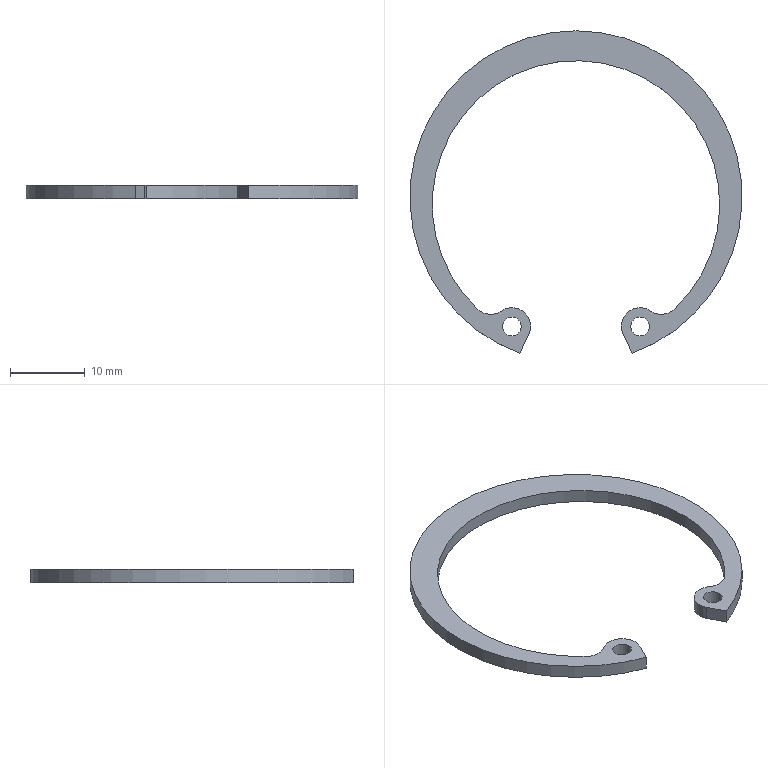Part | STEP file | KS B 1336 - 42x1.8 | 1 solid | 16 faces | box 44.5 x 43.174 x 1.8 mm | volume 686.31 mm3 | cylinder 12 | plane 4 | commonest cylinder face diameters 2.5 x4 5 x4 38.5 x2 44.5 x2
STEP:
#1=CARTESIAN_POINT('',(0.,0.,0.));
#2=DIRECTION('',(0.,0.,1.));
#3=DIRECTION('',(1.,0.,0.));
#4=AXIS2_PLACEMENT_3D('',#1,#2,#3);
#5=CARTESIAN_POINT('',(7.332,-38.343,0.));
#6=VERTEX_POINT('',#5);
#7=CARTESIAN_POINT('',(7.332,-38.343,1.8));
#8=VERTEX_POINT('',#7);
#9=CARTESIAN_POINT('',(7.332,-38.343,0.));
#10=DIRECTION('',(0.,0.,1.));
#11=VECTOR('',#10,1.);
#12=LINE('',#9,#11);
#13=CARTESIAN_POINT('',(8.582,-38.343,0.));
#14=DIRECTION('',(0.,0.,1.));
#15=DIRECTION('',(-1.,0.,0.));
#16=AXIS2_PLACEMENT_3D('',#13,#14,#15);
#17=CYLINDRICAL_SURFACE('',#16,1.25);
#18=CARTESIAN_POINT('',(6.283,0.));
#19=DIRECTION('',(0.,1.));
#20=VECTOR('',#19,1.);
#21=LINE('',#18,#20);
#22=(GEOMETRIC_REPRESENTATION_CONTEXT(2)PARAMETRIC_REPRESENTATION_CONTEXT()REPRESENTATION_CONTEXT('',''));
#23=DEFINITIONAL_REPRESENTATION('',(#21),#22);
#24=PCURVE('',#17,#23);
#25=CARTESIAN_POINT('',(8.582,-38.343,0.));
#26=DIRECTION('',(0.,0.,1.));
#27=DIRECTION('',(-1.,0.,0.));
#28=AXIS2_PLACEMENT_3D('',#25,#26,#27);
#29=CYLINDRICAL_SURFACE('',#28,1.25);
#30=CARTESIAN_POINT('',(0.,0.));
#31=DIRECTION('',(0.,1.));
#32=VECTOR('',#31,1.);
#33=LINE('',#30,#32);
#34=(GEOMETRIC_REPRESENTATION_CONTEXT(2)PARAMETRIC_REPRESENTATION_CONTEXT()REPRESENTATION_CONTEXT('',''));
#35=DEFINITIONAL_REPRESENTATION('',(#33),#34);
#36=PCURVE('',#29,#35);
#37=SURFACE_CURVE('',#12,(#24,#36),.PCURVE_S1.);
#38=EDGE_CURVE('',#6,#8,#37,.T.);
#39=ORIENTED_EDGE('',*,*,#38,.T.);
#40=CARTESIAN_POINT('',(9.832,-38.343,1.8));
#41=VERTEX_POINT('',#40);
#42=CARTESIAN_POINT('',(8.582,-38.343,1.8));
#43=DIRECTION('',(0.,0.,-1.));
#44=DIRECTION('',(-1.,0.,0.));
#45=AXIS2_PLACEMENT_3D('',#42,#43,#44);
#46=CIRCLE('',#45,1.25);
#47=CARTESIAN_POINT('',(6.283,1.8));
#48=DIRECTION('',(-1.,0.));
#49=VECTOR('',#48,1.);
#50=LINE('',#47,#49);
#51=(GEOMETRIC_REPRESENTATION_CONTEXT(2)PARAMETRIC_REPRESENTATION_CONTEXT()REPRESENTATION_CONTEXT('',''));
#52=DEFINITIONAL_REPRESENTATION('',(#50),#51);
#53=PCURVE('',#17,#52);
#54=CARTESIAN_POINT('',(-0.06301,-20.884,1.8));
#55=DIRECTION('',(0.,0.,1.));
#56=DIRECTION('',(1.,0.,0.));
#57=AXIS2_PLACEMENT_3D('',#54,#55,#56);
#58=PLANE('',#57);
#59=CARTESIAN_POINT('',(7.395,-17.459));
#60=CARTESIAN_POINT('',(7.395,-15.294));
#61=CARTESIAN_POINT('',(9.27,-16.376));
#62=CARTESIAN_POINT('',(11.145,-17.459));
#63=CARTESIAN_POINT('',(9.27,-18.541));
#64=CARTESIAN_POINT('',(7.395,-19.624));
#65=CARTESIAN_POINT('',(7.395,-17.459));
#66=(BOUNDED_CURVE()B_SPLINE_CURVE(2,(#59,#60,#61,#62,#63,#64,#65),.UNSPECIFIED.,.T.,.F.)B_SPLINE_CURVE_WITH_KNOTS((1,2,2,2,2,1),(-2.094,0.,2.094,4.189,6.283,8.378),.UNSPECIFIED.)CURVE()GEOMETRIC_REPRESENTATION_ITEM()RATIONAL_B_SPLINE_CURVE((1.,0.5,1.,0.5,1.,0.5,1.))REPRESENTATION_ITEM(''));
#67=(GEOMETRIC_REPRESENTATION_CONTEXT(2)PARAMETRIC_REPRESENTATION_CONTEXT()REPRESENTATION_CONTEXT('',''));
#68=DEFINITIONAL_REPRESENTATION('',(#66),#67);
#69=PCURVE('',#58,#68);
#70=SURFACE_CURVE('',#46,(#53,#69),.PCURVE_S1.);
#71=EDGE_CURVE('',#8,#41,#70,.T.);
#72=ORIENTED_EDGE('',*,*,#71,.T.);
#73=CARTESIAN_POINT('',(9.832,-38.343,0.));
#74=VERTEX_POINT('',#73);
#75=CARTESIAN_POINT('',(9.832,-38.343,0.));
#76=DIRECTION('',(0.,0.,1.));
#77=VECTOR('',#76,1.);
#78=LINE('',#75,#77);
#79=CARTESIAN_POINT('',(3.142,0.));
#80=DIRECTION('',(0.,1.));
#81=VECTOR('',#80,1.);
#82=LINE('',#79,#81);
#83=(GEOMETRIC_REPRESENTATION_CONTEXT(2)PARAMETRIC_REPRESENTATION_CONTEXT()REPRESENTATION_CONTEXT('',''));
#84=DEFINITIONAL_REPRESENTATION('',(#82),#83);
#85=PCURVE('',#17,#84);
#86=CARTESIAN_POINT('',(3.142,0.));
#87=DIRECTION('',(0.,1.));
#88=VECTOR('',#87,1.);
#89=LINE('',#86,#88);
#90=(GEOMETRIC_REPRESENTATION_CONTEXT(2)PARAMETRIC_REPRESENTATION_CONTEXT()REPRESENTATION_CONTEXT('',''));
#91=DEFINITIONAL_REPRESENTATION('',(#89),#90);
#92=PCURVE('',#29,#91);
#93=SURFACE_CURVE('',#78,(#85,#92),.PCURVE_S1.);
#94=EDGE_CURVE('',#74,#41,#93,.T.);
#95=ORIENTED_EDGE('',*,*,#94,.F.);
#96=CARTESIAN_POINT('',(8.582,-38.343,0.));
#97=DIRECTION('',(0.,0.,1.));
#98=DIRECTION('',(-1.,0.,0.));
#99=AXIS2_PLACEMENT_3D('',#96,#97,#98);
#100=CIRCLE('',#99,1.25);
#101=CARTESIAN_POINT('',(0.,0.));
#102=DIRECTION('',(1.,0.));
#103=VECTOR('',#102,1.);
#104=LINE('',#101,#103);
#105=(GEOMETRIC_REPRESENTATION_CONTEXT(2)PARAMETRIC_REPRESENTATION_CONTEXT()REPRESENTATION_CONTEXT('',''));
#106=DEFINITIONAL_REPRESENTATION('',(#104),#105);
#107=PCURVE('',#17,#106);
#108=CARTESIAN_POINT('',(-0.06301,-20.884,0.));
#109=DIRECTION('',(0.,0.,1.));
#110=DIRECTION('',(1.,0.,0.));
#111=AXIS2_PLACEMENT_3D('',#108,#109,#110);
#112=PLANE('',#111);
#113=CARTESIAN_POINT('',(8.645,-17.459));
#114=DIRECTION('',(-1.,0.));
#115=AXIS2_PLACEMENT_2D('',#113,#114);
#116=CIRCLE('',#115,1.25);
#117=(GEOMETRIC_REPRESENTATION_CONTEXT(2)PARAMETRIC_REPRESENTATION_CONTEXT()REPRESENTATION_CONTEXT('',''));
#118=DEFINITIONAL_REPRESENTATION('',(#116),#117);
#119=PCURVE('',#112,#118);
#120=SURFACE_CURVE('',#100,(#107,#119),.PCURVE_S1.);
#121=EDGE_CURVE('',#74,#6,#120,.T.);
#122=ORIENTED_EDGE('',*,*,#121,.T.);
#123=EDGE_LOOP('',(#39,#72,#95,#122));
#124=FACE_BOUND('',#123,.F.);
#125=ADVANCED_FACE('',(#124),#17,.F.);
#126=CARTESIAN_POINT('',(-9.832,-38.343,0.));
#127=VERTEX_POINT('',#126);
#128=CARTESIAN_POINT('',(-9.832,-38.343,1.8));
#129=VERTEX_POINT('',#128);
#130=CARTESIAN_POINT('',(-9.832,-38.343,0.));
#131=DIRECTION('',(0.,0.,1.));
#132=VECTOR('',#131,1.);
#133=LINE('',#130,#132);
#134=CARTESIAN_POINT('',(-8.582,-38.343,0.));
#135=DIRECTION('',(0.,0.,1.));
#136=DIRECTION('',(-1.,0.,0.));
#137=AXIS2_PLACEMENT_3D('',#134,#135,#136);
#138=CYLINDRICAL_SURFACE('',#137,1.25);
#139=CARTESIAN_POINT('',(6.283,0.));
#140=DIRECTION('',(0.,1.));
#141=VECTOR('',#140,1.);
#142=LINE('',#139,#141);
#143=(GEOMETRIC_REPRESENTATION_CONTEXT(2)PARAMETRIC_REPRESENTATION_CONTEXT()REPRESENTATION_CONTEXT('',''));
#144=DEFINITIONAL_REPRESENTATION('',(#142),#143);
#145=PCURVE('',#138,#144);
#146=CARTESIAN_POINT('',(-8.582,-38.343,0.));
#147=DIRECTION('',(0.,0.,1.));
#148=DIRECTION('',(-1.,0.,0.));
#149=AXIS2_PLACEMENT_3D('',#146,#147,#148);
#150=CYLINDRICAL_SURFACE('',#149,1.25);
#151=CARTESIAN_POINT('',(0.,0.));
#152=DIRECTION('',(0.,1.));
#153=VECTOR('',#152,1.);
#154=LINE('',#151,#153);
#155=(GEOMETRIC_REPRESENTATION_CONTEXT(2)PARAMETRIC_REPRESENTATION_CONTEXT()REPRESENTATION_CONTEXT('',''));
#156=DEFINITIONAL_REPRESENTATION('',(#154),#155);
#157=PCURVE('',#150,#156);
#158=SURFACE_CURVE('',#133,(#145,#157),.PCURVE_S1.);
#159=EDGE_CURVE('',#127,#129,#158,.T.);
#160=ORIENTED_EDGE('',*,*,#159,.T.);
#161=CARTESIAN_POINT('',(-7.332,-38.343,1.8));
#162=VERTEX_POINT('',#161);
#163=CARTESIAN_POINT('',(-8.582,-38.343,1.8));
#164=DIRECTION('',(0.,0.,-1.));
#165=DIRECTION('',(-1.,0.,0.));
#166=AXIS2_PLACEMENT_3D('',#163,#164,#165);
#167=CIRCLE('',#166,1.25);
#168=CARTESIAN_POINT('',(6.283,1.8));
#169=DIRECTION('',(-1.,0.));
#170=VECTOR('',#169,1.);
#171=LINE('',#168,#170);
#172=(GEOMETRIC_REPRESENTATION_CONTEXT(2)PARAMETRIC_REPRESENTATION_CONTEXT()REPRESENTATION_CONTEXT('',''));
#173=DEFINITIONAL_REPRESENTATION('',(#171),#172);
#174=PCURVE('',#138,#173);
#175=CARTESIAN_POINT('',(-9.769,-17.459));
#176=CARTESIAN_POINT('',(-9.769,-15.294));
#177=CARTESIAN_POINT('',(-7.894,-16.376));
#178=CARTESIAN_POINT('',(-6.019,-17.459));
#179=CARTESIAN_POINT('',(-7.894,-18.541));
#180=CARTESIAN_POINT('',(-9.769,-19.624));
#181=CARTESIAN_POINT('',(-9.769,-17.459));
#182=(BOUNDED_CURVE()B_SPLINE_CURVE(2,(#175,#176,#177,#178,#179,#180,#181),.UNSPECIFIED.,.T.,.F.)B_SPLINE_CURVE_WITH_KNOTS((1,2,2,2,2,1),(-2.094,0.,2.094,4.189,6.283,8.378),.UNSPECIFIED.)CURVE()GEOMETRIC_REPRESENTATION_ITEM()RATIONAL_B_SPLINE_CURVE((1.,0.5,1.,0.5,1.,0.5,1.))REPRESENTATION_ITEM(''));
#183=(GEOMETRIC_REPRESENTATION_CONTEXT(2)PARAMETRIC_REPRESENTATION_CONTEXT()REPRESENTATION_CONTEXT('',''));
#184=DEFINITIONAL_REPRESENTATION('',(#182),#183);
#185=PCURVE('',#58,#184);
#186=SURFACE_CURVE('',#167,(#174,#185),.PCURVE_S1.);
#187=EDGE_CURVE('',#129,#162,#186,.T.);
#188=ORIENTED_EDGE('',*,*,#187,.T.);
#189=CARTESIAN_POINT('',(-7.332,-38.343,0.));
#190=VERTEX_POINT('',#189);
#191=CARTESIAN_POINT('',(-7.332,-38.343,0.));
#192=DIRECTION('',(0.,0.,1.));
#193=VECTOR('',#192,1.);
#194=LINE('',#191,#193);
#195=CARTESIAN_POINT('',(3.142,0.));
#196=DIRECTION('',(0.,1.));
#197=VECTOR('',#196,1.);
#198=LINE('',#195,#197);
#199=(GEOMETRIC_REPRESENTATION_CONTEXT(2)PARAMETRIC_REPRESENTATION_CONTEXT()REPRESENTATION_CONTEXT('',''));
#200=DEFINITIONAL_REPRESENTATION('',(#198),#199);
#201=PCURVE('',#138,#200);
#202=CARTESIAN_POINT('',(3.142,0.));
#203=DIRECTION('',(0.,1.));
#204=VECTOR('',#203,1.);
#205=LINE('',#202,#204);
#206=(GEOMETRIC_REPRESENTATION_CONTEXT(2)PARAMETRIC_REPRESENTATION_CONTEXT()REPRESENTATION_CONTEXT('',''));
#207=DEFINITIONAL_REPRESENTATION('',(#205),#206);
#208=PCURVE('',#150,#207);
#209=SURFACE_CURVE('',#194,(#201,#208),.PCURVE_S1.);
#210=EDGE_CURVE('',#190,#162,#209,.T.);
#211=ORIENTED_EDGE('',*,*,#210,.F.);
#212=CARTESIAN_POINT('',(-8.582,-38.343,0.));
#213=DIRECTION('',(0.,0.,1.));
#214=DIRECTION('',(-1.,0.,0.));
#215=AXIS2_PLACEMENT_3D('',#212,#213,#214);
#216=CIRCLE('',#215,1.25);
#217=CARTESIAN_POINT('',(0.,0.));
#218=DIRECTION('',(1.,0.));
#219=VECTOR('',#218,1.);
#220=LINE('',#217,#219);
#221=(GEOMETRIC_REPRESENTATION_CONTEXT(2)PARAMETRIC_REPRESENTATION_CONTEXT()REPRESENTATION_CONTEXT('',''));
#222=DEFINITIONAL_REPRESENTATION('',(#220),#221);
#223=PCURVE('',#138,#222);
#224=CARTESIAN_POINT('',(-8.519,-17.459));
#225=DIRECTION('',(-1.,0.));
#226=AXIS2_PLACEMENT_2D('',#224,#225);
#227=CIRCLE('',#226,1.25);
#228=(GEOMETRIC_REPRESENTATION_CONTEXT(2)PARAMETRIC_REPRESENTATION_CONTEXT()REPRESENTATION_CONTEXT('',''));
#229=DEFINITIONAL_REPRESENTATION('',(#227),#228);
#230=PCURVE('',#112,#229);
#231=SURFACE_CURVE('',#216,(#223,#230),.PCURVE_S1.);
#232=EDGE_CURVE('',#190,#127,#231,.T.);
#233=ORIENTED_EDGE('',*,*,#232,.T.);
#234=EDGE_LOOP('',(#160,#188,#211,#233));
#235=FACE_BOUND('',#234,.F.);
#236=ADVANCED_FACE('',(#235),#138,.F.);
#237=CARTESIAN_POINT('',(-13.144,-36.064,0.));
#238=VERTEX_POINT('',#237);
#239=CARTESIAN_POINT('',(-13.144,-36.064,1.8));
#240=VERTEX_POINT('',#239);
#241=CARTESIAN_POINT('',(-13.144,-36.064,0.));
#242=DIRECTION('',(0.,0.,1.));
#243=VECTOR('',#242,1.);
#244=LINE('',#241,#243);
#245=CARTESIAN_POINT('',(0.,-22.,0.));
#246=DIRECTION('',(0.,0.,1.));
#247=DIRECTION('',(-0.6828,0.7306,0.));
#248=AXIS2_PLACEMENT_3D('',#245,#246,#247);
#249=CYLINDRICAL_SURFACE('',#248,19.25);
#250=CARTESIAN_POINT('',(1.638,0.));
#251=DIRECTION('',(0.,1.));
#252=VECTOR('',#251,1.);
#253=LINE('',#250,#252);
#254=(GEOMETRIC_REPRESENTATION_CONTEXT(2)PARAMETRIC_REPRESENTATION_CONTEXT()REPRESENTATION_CONTEXT('',''));
#255=DEFINITIONAL_REPRESENTATION('',(#253),#254);
#256=PCURVE('',#249,#255);
#257=CARTESIAN_POINT('',(-11.437,-34.238,0.));
#258=DIRECTION('',(0.,0.,1.));
#259=DIRECTION('',(0.6828,0.7306,0.));
#260=AXIS2_PLACEMENT_3D('',#257,#258,#259);
#261=CYLINDRICAL_SURFACE('',#260,2.5);
#262=CARTESIAN_POINT('',(3.142,0.));
#263=DIRECTION('',(0.,1.));
#264=VECTOR('',#263,1.);
#265=LINE('',#262,#264);
#266=(GEOMETRIC_REPRESENTATION_CONTEXT(2)PARAMETRIC_REPRESENTATION_CONTEXT()REPRESENTATION_CONTEXT('',''));
#267=DEFINITIONAL_REPRESENTATION('',(#265),#266);
#268=PCURVE('',#261,#267);
#269=SURFACE_CURVE('',#244,(#256,#268),.PCURVE_S1.);
#270=EDGE_CURVE('',#238,#240,#269,.T.);
#271=ORIENTED_EDGE('',*,*,#270,.T.);
#272=CARTESIAN_POINT('',(-13.144,-7.936,1.8));
#273=VERTEX_POINT('',#272);
#274=CARTESIAN_POINT('',(0.,-22.,1.8));
#275=DIRECTION('',(0.,0.,1.));
#276=DIRECTION('',(-0.6828,0.7306,0.));
#277=AXIS2_PLACEMENT_3D('',#274,#275,#276);
#278=CIRCLE('',#277,19.25);
#279=CARTESIAN_POINT('',(0.,1.8));
#280=DIRECTION('',(1.,0.));
#281=VECTOR('',#280,1.);
#282=LINE('',#279,#281);
#283=(GEOMETRIC_REPRESENTATION_CONTEXT(2)PARAMETRIC_REPRESENTATION_CONTEXT()REPRESENTATION_CONTEXT('',''));
#284=DEFINITIONAL_REPRESENTATION('',(#282),#283);
#285=PCURVE('',#249,#284);
#286=CARTESIAN_POINT('',(0.06301,-1.116));
#287=DIRECTION('',(-0.6828,0.7306));
#288=AXIS2_PLACEMENT_2D('',#286,#287);
#289=CIRCLE('',#288,19.25);
#290=(GEOMETRIC_REPRESENTATION_CONTEXT(2)PARAMETRIC_REPRESENTATION_CONTEXT()REPRESENTATION_CONTEXT('',''));
#291=DEFINITIONAL_REPRESENTATION('',(#289),#290);
#292=PCURVE('',#58,#291);
#293=SURFACE_CURVE('',#278,(#285,#292),.PCURVE_S1.);
#294=EDGE_CURVE('',#273,#240,#293,.T.);
#295=ORIENTED_EDGE('',*,*,#294,.F.);
#296=CARTESIAN_POINT('',(-13.144,-7.936,0.));
#297=VERTEX_POINT('',#296);
#298=CARTESIAN_POINT('',(-13.144,-7.936,0.));
#299=DIRECTION('',(0.,0.,1.));
#300=VECTOR('',#299,1.);
#301=LINE('',#298,#300);
#302=CARTESIAN_POINT('',(0.,0.));
#303=DIRECTION('',(0.,1.));
#304=VECTOR('',#303,1.);
#305=LINE('',#302,#304);
#306=(GEOMETRIC_REPRESENTATION_CONTEXT(2)PARAMETRIC_REPRESENTATION_CONTEXT()REPRESENTATION_CONTEXT('',''));
#307=DEFINITIONAL_REPRESENTATION('',(#305),#306);
#308=PCURVE('',#249,#307);
#309=CARTESIAN_POINT('',(0.,-22.,0.));
#310=DIRECTION('',(0.,0.,1.));
#311=DIRECTION('',(-0.6828,0.7306,0.));
#312=AXIS2_PLACEMENT_3D('',#309,#310,#311);
#313=CYLINDRICAL_SURFACE('',#312,19.25);
#314=CARTESIAN_POINT('',(6.283,0.));
#315=DIRECTION('',(0.,1.));
#316=VECTOR('',#315,1.);
#317=LINE('',#314,#316);
#318=(GEOMETRIC_REPRESENTATION_CONTEXT(2)PARAMETRIC_REPRESENTATION_CONTEXT()REPRESENTATION_CONTEXT('',''));
#319=DEFINITIONAL_REPRESENTATION('',(#317),#318);
#320=PCURVE('',#313,#319);
#321=SURFACE_CURVE('',#301,(#308,#320),.PCURVE_S1.);
#322=EDGE_CURVE('',#297,#273,#321,.T.);
#323=ORIENTED_EDGE('',*,*,#322,.F.);
#324=CARTESIAN_POINT('',(0.,-22.,0.));
#325=DIRECTION('',(0.,0.,-1.));
#326=DIRECTION('',(-0.6828,0.7306,0.));
#327=AXIS2_PLACEMENT_3D('',#324,#325,#326);
#328=CIRCLE('',#327,19.25);
#329=CARTESIAN_POINT('',(6.283,0.));
#330=DIRECTION('',(-1.,0.));
#331=VECTOR('',#330,1.);
#332=LINE('',#329,#331);
#333=(GEOMETRIC_REPRESENTATION_CONTEXT(2)PARAMETRIC_REPRESENTATION_CONTEXT()REPRESENTATION_CONTEXT('',''));
#334=DEFINITIONAL_REPRESENTATION('',(#332),#333);
#335=PCURVE('',#249,#334);
#336=CARTESIAN_POINT('',(-13.081,12.948));
#337=CARTESIAN_POINT('',(11.28,35.714));
#338=CARTESIAN_POINT('',(18.815,3.235));
#339=CARTESIAN_POINT('',(26.35,-29.245));
#340=CARTESIAN_POINT('',(-5.545,-19.531));
#341=CARTESIAN_POINT('',(-37.441,-9.817));
#342=CARTESIAN_POINT('',(-13.081,12.948));
#343=(BOUNDED_CURVE()B_SPLINE_CURVE(2,(#336,#337,#338,#339,#340,#341,#342),.UNSPECIFIED.,.T.,.F.)B_SPLINE_CURVE_WITH_KNOTS((1,2,2,2,2,1),(-2.094,0.,2.094,4.189,6.283,8.378),.UNSPECIFIED.)CURVE()GEOMETRIC_REPRESENTATION_ITEM()RATIONAL_B_SPLINE_CURVE((1.,0.5,1.,0.5,1.,0.5,1.))REPRESENTATION_ITEM(''));
#344=(GEOMETRIC_REPRESENTATION_CONTEXT(2)PARAMETRIC_REPRESENTATION_CONTEXT()REPRESENTATION_CONTEXT('',''));
#345=DEFINITIONAL_REPRESENTATION('',(#343),#344);
#346=PCURVE('',#112,#345);
#347=SURFACE_CURVE('',#328,(#335,#346),.PCURVE_S1.);
#348=EDGE_CURVE('',#238,#297,#347,.T.);
#349=ORIENTED_EDGE('',*,*,#348,.F.);
#350=EDGE_LOOP('',(#271,#295,#323,#349));
#351=FACE_BOUND('',#350,.F.);
#352=ADVANCED_FACE('',(#351),#249,.F.);
#353=CARTESIAN_POINT('',(7.565,-41.924,0.));
#354=VERTEX_POINT('',#353);
#355=CARTESIAN_POINT('',(0.,1.25,0.));
#356=VERTEX_POINT('',#355);
#357=CARTESIAN_POINT('',(0.,-21.,0.));
#358=DIRECTION('',(0.,0.,1.));
#359=DIRECTION('',(0.34,-0.9404,0.));
#360=AXIS2_PLACEMENT_3D('',#357,#358,#359);
#361=CIRCLE('',#360,22.25);
#362=CARTESIAN_POINT('',(0.,-21.,0.));
#363=DIRECTION('',(0.,0.,1.));
#364=DIRECTION('',(0.,1.,0.));
#365=AXIS2_PLACEMENT_3D('',#362,#363,#364);
#366=CYLINDRICAL_SURFACE('',#365,22.25);
#367=CARTESIAN_POINT('',(3.489,0.));
#368=DIRECTION('',(1.,0.));
#369=VECTOR('',#368,1.);
#370=LINE('',#367,#369);
#371=(GEOMETRIC_REPRESENTATION_CONTEXT(2)PARAMETRIC_REPRESENTATION_CONTEXT()REPRESENTATION_CONTEXT('',''));
#372=DEFINITIONAL_REPRESENTATION('',(#370),#371);
#373=PCURVE('',#366,#372);
#374=CARTESIAN_POINT('',(0.06301,-0.1159));
#375=DIRECTION('',(0.34,-0.9404));
#376=AXIS2_PLACEMENT_2D('',#374,#375);
#377=CIRCLE('',#376,22.25);
#378=(GEOMETRIC_REPRESENTATION_CONTEXT(2)PARAMETRIC_REPRESENTATION_CONTEXT()REPRESENTATION_CONTEXT('',''));
#379=DEFINITIONAL_REPRESENTATION('',(#377),#378);
#380=PCURVE('',#112,#379);
#381=SURFACE_CURVE('',#361,(#373,#380),.PCURVE_S1.);
#382=EDGE_CURVE('',#354,#356,#381,.T.);
#383=ORIENTED_EDGE('',*,*,#382,.T.);
#384=CARTESIAN_POINT('',(0.,1.25,1.8));
#385=VERTEX_POINT('',#384);
#386=CARTESIAN_POINT('',(0.,1.25,0.));
#387=DIRECTION('',(0.,0.,1.));
#388=VECTOR('',#387,1.);
#389=LINE('',#386,#388);
#390=CARTESIAN_POINT('',(6.283,0.));
#391=DIRECTION('',(0.,1.));
#392=VECTOR('',#391,1.);
#393=LINE('',#390,#392);
#394=(GEOMETRIC_REPRESENTATION_CONTEXT(2)PARAMETRIC_REPRESENTATION_CONTEXT()REPRESENTATION_CONTEXT('',''));
#395=DEFINITIONAL_REPRESENTATION('',(#393),#394);
#396=PCURVE('',#366,#395);
#397=CARTESIAN_POINT('',(0.,-21.,0.));
#398=DIRECTION('',(0.,0.,1.));
#399=DIRECTION('',(0.,1.,0.));
#400=AXIS2_PLACEMENT_3D('',#397,#398,#399);
#401=CYLINDRICAL_SURFACE('',#400,22.25);
#402=CARTESIAN_POINT('',(0.,0.));
#403=DIRECTION('',(0.,1.));
#404=VECTOR('',#403,1.);
#405=LINE('',#402,#404);
#406=(GEOMETRIC_REPRESENTATION_CONTEXT(2)PARAMETRIC_REPRESENTATION_CONTEXT()REPRESENTATION_CONTEXT('',''));
#407=DEFINITIONAL_REPRESENTATION('',(#405),#406);
#408=PCURVE('',#401,#407);
#409=SURFACE_CURVE('',#389,(#396,#408),.PCURVE_S1.);
#410=EDGE_CURVE('',#356,#385,#409,.T.);
#411=ORIENTED_EDGE('',*,*,#410,.T.);
#412=CARTESIAN_POINT('',(7.565,-41.924,1.8));
#413=VERTEX_POINT('',#412);
#414=CARTESIAN_POINT('',(0.,-21.,1.8));
#415=DIRECTION('',(0.,0.,-1.));
#416=DIRECTION('',(0.34,-0.9404,0.));
#417=AXIS2_PLACEMENT_3D('',#414,#415,#416);
#418=CIRCLE('',#417,22.25);
#419=CARTESIAN_POINT('',(9.772,1.8));
#420=DIRECTION('',(-1.,0.));
#421=VECTOR('',#420,1.);
#422=LINE('',#419,#421);
#423=(GEOMETRIC_REPRESENTATION_CONTEXT(2)PARAMETRIC_REPRESENTATION_CONTEXT()REPRESENTATION_CONTEXT('',''));
#424=DEFINITIONAL_REPRESENTATION('',(#422),#423);
#425=PCURVE('',#366,#424);
#426=CARTESIAN_POINT('',(7.628,-21.04));
#427=CARTESIAN_POINT('',(-28.614,-34.143));
#428=CARTESIAN_POINT('',(-21.841,3.795));
#429=CARTESIAN_POINT('',(-15.067,41.733));
#430=CARTESIAN_POINT('',(14.402,16.898));
#431=CARTESIAN_POINT('',(43.87,-7.937));
#432=CARTESIAN_POINT('',(7.628,-21.04));
#433=(BOUNDED_CURVE()B_SPLINE_CURVE(2,(#426,#427,#428,#429,#430,#431,#432),.UNSPECIFIED.,.T.,.F.)B_SPLINE_CURVE_WITH_KNOTS((1,2,2,2,2,1),(-2.094,0.,2.094,4.189,6.283,8.378),.UNSPECIFIED.)CURVE()GEOMETRIC_REPRESENTATION_ITEM()RATIONAL_B_SPLINE_CURVE((1.,0.5,1.,0.5,1.,0.5,1.))REPRESENTATION_ITEM(''));
#434=(GEOMETRIC_REPRESENTATION_CONTEXT(2)PARAMETRIC_REPRESENTATION_CONTEXT()REPRESENTATION_CONTEXT('',''));
#435=DEFINITIONAL_REPRESENTATION('',(#433),#434);
#436=PCURVE('',#58,#435);
#437=SURFACE_CURVE('',#418,(#425,#436),.PCURVE_S1.);
#438=EDGE_CURVE('',#385,#413,#437,.T.);
#439=ORIENTED_EDGE('',*,*,#438,.T.);
#440=CARTESIAN_POINT('',(7.565,-41.924,0.));
#441=DIRECTION('',(0.,0.,1.));
#442=VECTOR('',#441,1.);
#443=LINE('',#440,#442);
#444=CARTESIAN_POINT('',(3.489,0.));
#445=DIRECTION('',(0.,1.));
#446=VECTOR('',#445,1.);
#447=LINE('',#444,#446);
#448=(GEOMETRIC_REPRESENTATION_CONTEXT(2)PARAMETRIC_REPRESENTATION_CONTEXT()REPRESENTATION_CONTEXT('',''));
#449=DEFINITIONAL_REPRESENTATION('',(#447),#448);
#450=PCURVE('',#366,#449);
#451=CARTESIAN_POINT('',(7.565,-41.924,0.));
#452=DIRECTION('',(-0.8963,-0.4435,0.));
#453=DIRECTION('',(-0.4435,0.8963,0.));
#454=AXIS2_PLACEMENT_3D('',#451,#452,#453);
#455=PLANE('',#454);
#456=CARTESIAN_POINT('',(0.,0.));
#457=DIRECTION('',(0.,-1.));
#458=VECTOR('',#457,1.);
#459=LINE('',#456,#458);
#460=(GEOMETRIC_REPRESENTATION_CONTEXT(2)PARAMETRIC_REPRESENTATION_CONTEXT()REPRESENTATION_CONTEXT('',''));
#461=DEFINITIONAL_REPRESENTATION('',(#459),#460);
#462=PCURVE('',#455,#461);
#463=SURFACE_CURVE('',#443,(#450,#462),.PCURVE_S1.);
#464=EDGE_CURVE('',#354,#413,#463,.T.);
#465=ORIENTED_EDGE('',*,*,#464,.F.);
#466=EDGE_LOOP('',(#383,#411,#439,#465));
#467=FACE_BOUND('',#466,.T.);
#468=ADVANCED_FACE('',(#467),#366,.T.);
#469=ORIENTED_EDGE('',*,*,#187,.T.);
#470=CARTESIAN_POINT('',(-8.582,-38.343,1.8));
#471=DIRECTION('',(0.,0.,-1.));
#472=DIRECTION('',(-1.,0.,0.));
#473=AXIS2_PLACEMENT_3D('',#470,#471,#472);
#474=CIRCLE('',#473,1.25);
#475=CARTESIAN_POINT('',(-9.769,-17.459));
#476=CARTESIAN_POINT('',(-9.769,-15.294));
#477=CARTESIAN_POINT('',(-7.894,-16.376));
#478=CARTESIAN_POINT('',(-6.019,-17.459));
#479=CARTESIAN_POINT('',(-7.894,-18.541));
#480=CARTESIAN_POINT('',(-9.769,-19.624));
#481=CARTESIAN_POINT('',(-9.769,-17.459));
#482=(BOUNDED_CURVE()B_SPLINE_CURVE(2,(#475,#476,#477,#478,#479,#480,#481),.UNSPECIFIED.,.T.,.F.)B_SPLINE_CURVE_WITH_KNOTS((1,2,2,2,2,1),(-2.094,0.,2.094,4.189,6.283,8.378),.UNSPECIFIED.)CURVE()GEOMETRIC_REPRESENTATION_ITEM()RATIONAL_B_SPLINE_CURVE((1.,0.5,1.,0.5,1.,0.5,1.))REPRESENTATION_ITEM(''));
#483=(GEOMETRIC_REPRESENTATION_CONTEXT(2)PARAMETRIC_REPRESENTATION_CONTEXT()REPRESENTATION_CONTEXT('',''));
#484=DEFINITIONAL_REPRESENTATION('',(#482),#483);
#485=PCURVE('',#58,#484);
#486=CARTESIAN_POINT('',(6.283,1.8));
#487=DIRECTION('',(-1.,0.));
#488=VECTOR('',#487,1.);
#489=LINE('',#486,#488);
#490=(GEOMETRIC_REPRESENTATION_CONTEXT(2)PARAMETRIC_REPRESENTATION_CONTEXT()REPRESENTATION_CONTEXT('',''));
#491=DEFINITIONAL_REPRESENTATION('',(#489),#490);
#492=PCURVE('',#150,#491);
#493=SURFACE_CURVE('',#474,(#485,#492),.PCURVE_S1.);
#494=EDGE_CURVE('',#162,#129,#493,.T.);
#495=ORIENTED_EDGE('',*,*,#494,.T.);
#496=EDGE_LOOP('',(#469,#495));
#497=FACE_BOUND('',#496,.T.);
#498=ORIENTED_EDGE('',*,*,#71,.T.);
#499=CARTESIAN_POINT('',(8.582,-38.343,1.8));
#500=DIRECTION('',(0.,0.,-1.));
#501=DIRECTION('',(-1.,0.,0.));
#502=AXIS2_PLACEMENT_3D('',#499,#500,#501);
#503=CIRCLE('',#502,1.25);
#504=CARTESIAN_POINT('',(7.395,-17.459));
#505=CARTESIAN_POINT('',(7.395,-15.294));
#506=CARTESIAN_POINT('',(9.27,-16.376));
#507=CARTESIAN_POINT('',(11.145,-17.459));
#508=CARTESIAN_POINT('',(9.27,-18.541));
#509=CARTESIAN_POINT('',(7.395,-19.624));
#510=CARTESIAN_POINT('',(7.395,-17.459));
#511=(BOUNDED_CURVE()B_SPLINE_CURVE(2,(#504,#505,#506,#507,#508,#509,#510),.UNSPECIFIED.,.T.,.F.)B_SPLINE_CURVE_WITH_KNOTS((1,2,2,2,2,1),(-2.094,0.,2.094,4.189,6.283,8.378),.UNSPECIFIED.)CURVE()GEOMETRIC_REPRESENTATION_ITEM()RATIONAL_B_SPLINE_CURVE((1.,0.5,1.,0.5,1.,0.5,1.))REPRESENTATION_ITEM(''));
#512=(GEOMETRIC_REPRESENTATION_CONTEXT(2)PARAMETRIC_REPRESENTATION_CONTEXT()REPRESENTATION_CONTEXT('',''));
#513=DEFINITIONAL_REPRESENTATION('',(#511),#512);
#514=PCURVE('',#58,#513);
#515=CARTESIAN_POINT('',(6.283,1.8));
#516=DIRECTION('',(-1.,0.));
#517=VECTOR('',#516,1.);
#518=LINE('',#515,#517);
#519=(GEOMETRIC_REPRESENTATION_CONTEXT(2)PARAMETRIC_REPRESENTATION_CONTEXT()REPRESENTATION_CONTEXT('',''));
#520=DEFINITIONAL_REPRESENTATION('',(#518),#519);
#521=PCURVE('',#29,#520);
#522=SURFACE_CURVE('',#503,(#514,#521),.PCURVE_S1.);
#523=EDGE_CURVE('',#41,#8,#522,.T.);
#524=ORIENTED_EDGE('',*,*,#523,.T.);
#525=EDGE_LOOP('',(#498,#524));
#526=FACE_BOUND('',#525,.T.);
#527=CARTESIAN_POINT('',(13.144,-36.064,1.8));
#528=VERTEX_POINT('',#527);
#529=CARTESIAN_POINT('',(0.,-22.,1.8));
#530=DIRECTION('',(0.,0.,1.));
#531=DIRECTION('',(-0.6828,0.7306,0.));
#532=AXIS2_PLACEMENT_3D('',#529,#530,#531);
#533=CIRCLE('',#532,19.25);
#534=CARTESIAN_POINT('',(0.06301,-1.116));
#535=DIRECTION('',(-0.6828,0.7306));
#536=AXIS2_PLACEMENT_2D('',#534,#535);
#537=CIRCLE('',#536,19.25);
#538=(GEOMETRIC_REPRESENTATION_CONTEXT(2)PARAMETRIC_REPRESENTATION_CONTEXT()REPRESENTATION_CONTEXT('',''));
#539=DEFINITIONAL_REPRESENTATION('',(#537),#538);
#540=PCURVE('',#58,#539);
#541=CARTESIAN_POINT('',(0.,1.8));
#542=DIRECTION('',(1.,0.));
#543=VECTOR('',#542,1.);
#544=LINE('',#541,#543);
#545=(GEOMETRIC_REPRESENTATION_CONTEXT(2)PARAMETRIC_REPRESENTATION_CONTEXT()REPRESENTATION_CONTEXT('',''));
#546=DEFINITIONAL_REPRESENTATION('',(#544),#545);
#547=PCURVE('',#313,#546);
#548=SURFACE_CURVE('',#533,(#540,#547),.PCURVE_S1.);
#549=EDGE_CURVE('',#528,#273,#548,.T.);
#550=ORIENTED_EDGE('',*,*,#549,.F.);
#551=CARTESIAN_POINT('',(10.009,-36.29,1.8));
#552=VERTEX_POINT('',#551);
#553=CARTESIAN_POINT('',(11.437,-34.238,1.8));
#554=DIRECTION('',(0.,0.,1.));
#555=DIRECTION('',(0.5709,0.821,0.));
#556=AXIS2_PLACEMENT_3D('',#553,#554,#555);
#557=CIRCLE('',#556,2.5);
#558=CARTESIAN_POINT('',(11.5,-13.354));
#559=DIRECTION('',(0.5709,0.821));
#560=AXIS2_PLACEMENT_2D('',#558,#559);
#561=CIRCLE('',#560,2.5);
#562=(GEOMETRIC_REPRESENTATION_CONTEXT(2)PARAMETRIC_REPRESENTATION_CONTEXT()REPRESENTATION_CONTEXT('',''));
#563=DEFINITIONAL_REPRESENTATION('',(#561),#562);
#564=PCURVE('',#58,#563);
#565=CARTESIAN_POINT('',(11.437,-34.238,0.));
#566=DIRECTION('',(0.,0.,1.));
#567=DIRECTION('',(0.5709,0.821,0.));
#568=AXIS2_PLACEMENT_3D('',#565,#566,#567);
#569=CYLINDRICAL_SURFACE('',#568,2.5);
#570=CARTESIAN_POINT('',(0.,1.8));
#571=DIRECTION('',(1.,0.));
#572=VECTOR('',#571,1.);
#573=LINE('',#570,#572);
#574=(GEOMETRIC_REPRESENTATION_CONTEXT(2)PARAMETRIC_REPRESENTATION_CONTEXT()REPRESENTATION_CONTEXT('',''));
#575=DEFINITIONAL_REPRESENTATION('',(#573),#574);
#576=PCURVE('',#569,#575);
#577=SURFACE_CURVE('',#557,(#564,#576),.PCURVE_S1.);
#578=EDGE_CURVE('',#552,#528,#577,.T.);
#579=ORIENTED_EDGE('',*,*,#578,.F.);
#580=CARTESIAN_POINT('',(6.341,-39.452,1.8));
#581=VERTEX_POINT('',#580);
#582=CARTESIAN_POINT('',(8.582,-38.343,1.8));
#583=DIRECTION('',(0.,0.,-1.));
#584=DIRECTION('',(0.5709,0.821,0.));
#585=AXIS2_PLACEMENT_3D('',#582,#583,#584);
#586=CIRCLE('',#585,2.5);
#587=CARTESIAN_POINT('',(10.072,-15.406));
#588=CARTESIAN_POINT('',(13.627,-17.878));
#589=CARTESIAN_POINT('',(9.709,-19.721));
#590=CARTESIAN_POINT('',(5.79,-21.564));
#591=CARTESIAN_POINT('',(6.154,-17.249));
#592=CARTESIAN_POINT('',(6.517,-12.934));
#593=CARTESIAN_POINT('',(10.072,-15.406));
#594=(BOUNDED_CURVE()B_SPLINE_CURVE(2,(#587,#588,#589,#590,#591,#592,#593),.UNSPECIFIED.,.T.,.F.)B_SPLINE_CURVE_WITH_KNOTS((1,2,2,2,2,1),(-2.094,0.,2.094,4.189,6.283,8.378),.UNSPECIFIED.)CURVE()GEOMETRIC_REPRESENTATION_ITEM()RATIONAL_B_SPLINE_CURVE((1.,0.5,1.,0.5,1.,0.5,1.))REPRESENTATION_ITEM(''));
#595=(GEOMETRIC_REPRESENTATION_CONTEXT(2)PARAMETRIC_REPRESENTATION_CONTEXT()REPRESENTATION_CONTEXT('',''));
#596=DEFINITIONAL_REPRESENTATION('',(#594),#595);
#597=PCURVE('',#58,#596);
#598=CARTESIAN_POINT('',(8.582,-38.343,0.));
#599=DIRECTION('',(0.,0.,1.));
#600=DIRECTION('',(0.5709,0.821,0.));
#601=AXIS2_PLACEMENT_3D('',#598,#599,#600);
#602=CYLINDRICAL_SURFACE('',#601,2.5);
#603=CARTESIAN_POINT('',(6.283,1.8));
#604=DIRECTION('',(-1.,0.));
#605=VECTOR('',#604,1.);
#606=LINE('',#603,#605);
#607=(GEOMETRIC_REPRESENTATION_CONTEXT(2)PARAMETRIC_REPRESENTATION_CONTEXT()REPRESENTATION_CONTEXT('',''));
#608=DEFINITIONAL_REPRESENTATION('',(#606),#607);
#609=PCURVE('',#602,#608);
#610=SURFACE_CURVE('',#586,(#597,#609),.PCURVE_S1.);
#611=EDGE_CURVE('',#581,#552,#610,.T.);
#612=ORIENTED_EDGE('',*,*,#611,.F.);
#613=CARTESIAN_POINT('',(6.341,-39.452,1.8));
#614=DIRECTION('',(-0.4435,0.8963,0.));
#615=VECTOR('',#614,1.);
#616=LINE('',#613,#615);
#617=CARTESIAN_POINT('',(6.404,-18.567));
#618=DIRECTION('',(-0.4435,0.8963));
#619=VECTOR('',#618,1.);
#620=LINE('',#617,#619);
#621=(GEOMETRIC_REPRESENTATION_CONTEXT(2)PARAMETRIC_REPRESENTATION_CONTEXT()REPRESENTATION_CONTEXT('',''));
#622=DEFINITIONAL_REPRESENTATION('',(#620),#621);
#623=PCURVE('',#58,#622);
#624=CARTESIAN_POINT('',(2.759,-1.8));
#625=DIRECTION('',(1.,0.));
#626=VECTOR('',#625,1.);
#627=LINE('',#624,#626);
#628=(GEOMETRIC_REPRESENTATION_CONTEXT(2)PARAMETRIC_REPRESENTATION_CONTEXT()REPRESENTATION_CONTEXT('',''));
#629=DEFINITIONAL_REPRESENTATION('',(#627),#628);
#630=PCURVE('',#455,#629);
#631=SURFACE_CURVE('',#616,(#623,#630),.PCURVE_S1.);
#632=EDGE_CURVE('',#413,#581,#631,.T.);
#633=ORIENTED_EDGE('',*,*,#632,.F.);
#634=ORIENTED_EDGE('',*,*,#438,.F.);
#635=CARTESIAN_POINT('',(-7.565,-41.924,1.8));
#636=VERTEX_POINT('',#635);
#637=CARTESIAN_POINT('',(0.,-21.,1.8));
#638=DIRECTION('',(0.,0.,-1.));
#639=DIRECTION('',(0.34,-0.9404,0.));
#640=AXIS2_PLACEMENT_3D('',#637,#638,#639);
#641=CIRCLE('',#640,22.25);
#642=CARTESIAN_POINT('',(7.628,-21.04));
#643=CARTESIAN_POINT('',(-28.614,-34.143));
#644=CARTESIAN_POINT('',(-21.841,3.795));
#645=CARTESIAN_POINT('',(-15.067,41.733));
#646=CARTESIAN_POINT('',(14.402,16.898));
#647=CARTESIAN_POINT('',(43.87,-7.937));
#648=CARTESIAN_POINT('',(7.628,-21.04));
#649=(BOUNDED_CURVE()B_SPLINE_CURVE(2,(#642,#643,#644,#645,#646,#647,#648),.UNSPECIFIED.,.T.,.F.)B_SPLINE_CURVE_WITH_KNOTS((1,2,2,2,2,1),(-2.094,0.,2.094,4.189,6.283,8.378),.UNSPECIFIED.)CURVE()GEOMETRIC_REPRESENTATION_ITEM()RATIONAL_B_SPLINE_CURVE((1.,0.5,1.,0.5,1.,0.5,1.))REPRESENTATION_ITEM(''));
#650=(GEOMETRIC_REPRESENTATION_CONTEXT(2)PARAMETRIC_REPRESENTATION_CONTEXT()REPRESENTATION_CONTEXT('',''));
#651=DEFINITIONAL_REPRESENTATION('',(#649),#650);
#652=PCURVE('',#58,#651);
#653=CARTESIAN_POINT('',(3.489,1.8));
#654=DIRECTION('',(-1.,0.));
#655=VECTOR('',#654,1.);
#656=LINE('',#653,#655);
#657=(GEOMETRIC_REPRESENTATION_CONTEXT(2)PARAMETRIC_REPRESENTATION_CONTEXT()REPRESENTATION_CONTEXT('',''));
#658=DEFINITIONAL_REPRESENTATION('',(#656),#657);
#659=PCURVE('',#401,#658);
#660=SURFACE_CURVE('',#641,(#652,#659),.PCURVE_S1.);
#661=EDGE_CURVE('',#636,#385,#660,.T.);
#662=ORIENTED_EDGE('',*,*,#661,.F.);
#663=CARTESIAN_POINT('',(-6.341,-39.452,1.8));
#664=VERTEX_POINT('',#663);
#665=CARTESIAN_POINT('',(-7.565,-41.924,1.8));
#666=DIRECTION('',(-0.4435,-0.8963,0.));
#667=VECTOR('',#666,1.);
#668=LINE('',#665,#667);
#669=CARTESIAN_POINT('',(-7.502,-21.04));
#670=DIRECTION('',(-0.4435,-0.8963));
#671=VECTOR('',#670,1.);
#672=LINE('',#669,#671);
#673=(GEOMETRIC_REPRESENTATION_CONTEXT(2)PARAMETRIC_REPRESENTATION_CONTEXT()REPRESENTATION_CONTEXT('',''));
#674=DEFINITIONAL_REPRESENTATION('',(#672),#673);
#675=PCURVE('',#58,#674);
#676=CARTESIAN_POINT('',(-6.341,-39.452,0.));
#677=DIRECTION('',(0.8963,-0.4435,0.));
#678=DIRECTION('',(0.,0.,-1.));
#679=AXIS2_PLACEMENT_3D('',#676,#677,#678);
#680=PLANE('',#679);
#681=CARTESIAN_POINT('',(-1.8,-2.759));
#682=DIRECTION('',(0.,-1.));
#683=VECTOR('',#682,1.);
#684=LINE('',#681,#683);
#685=(GEOMETRIC_REPRESENTATION_CONTEXT(2)PARAMETRIC_REPRESENTATION_CONTEXT()REPRESENTATION_CONTEXT('',''));
#686=DEFINITIONAL_REPRESENTATION('',(#684),#685);
#687=PCURVE('',#680,#686);
#688=SURFACE_CURVE('',#668,(#675,#687),.PCURVE_S1.);
#689=EDGE_CURVE('',#664,#636,#688,.T.);
#690=ORIENTED_EDGE('',*,*,#689,.F.);
#691=CARTESIAN_POINT('',(-10.009,-36.29,1.8));
#692=VERTEX_POINT('',#691);
#693=CARTESIAN_POINT('',(-8.582,-38.343,1.8));
#694=DIRECTION('',(0.,0.,-1.));
#695=DIRECTION('',(0.8963,-0.4435,0.));
#696=AXIS2_PLACEMENT_3D('',#693,#694,#695);
#697=CIRCLE('',#696,2.5);
#698=CARTESIAN_POINT('',(-6.278,-18.567));
#699=CARTESIAN_POINT('',(-8.199,-22.448));
#700=CARTESIAN_POINT('',(-10.6,-18.845));
#701=CARTESIAN_POINT('',(-13.,-15.241));
#702=CARTESIAN_POINT('',(-8.679,-14.964));
#703=CARTESIAN_POINT('',(-4.358,-14.687));
#704=CARTESIAN_POINT('',(-6.278,-18.567));
#705=(BOUNDED_CURVE()B_SPLINE_CURVE(2,(#698,#699,#700,#701,#702,#703,#704),.UNSPECIFIED.,.T.,.F.)B_SPLINE_CURVE_WITH_KNOTS((1,2,2,2,2,1),(-2.094,0.,2.094,4.189,6.283,8.378),.UNSPECIFIED.)CURVE()GEOMETRIC_REPRESENTATION_ITEM()RATIONAL_B_SPLINE_CURVE((1.,0.5,1.,0.5,1.,0.5,1.))REPRESENTATION_ITEM(''));
#706=(GEOMETRIC_REPRESENTATION_CONTEXT(2)PARAMETRIC_REPRESENTATION_CONTEXT()REPRESENTATION_CONTEXT('',''));
#707=DEFINITIONAL_REPRESENTATION('',(#705),#706);
#708=PCURVE('',#58,#707);
#709=CARTESIAN_POINT('',(-8.582,-38.343,0.));
#710=DIRECTION('',(0.,0.,1.));
#711=DIRECTION('',(0.8963,-0.4435,0.));
#712=AXIS2_PLACEMENT_3D('',#709,#710,#711);
#713=CYLINDRICAL_SURFACE('',#712,2.5);
#714=CARTESIAN_POINT('',(6.283,1.8));
#715=DIRECTION('',(-1.,0.));
#716=VECTOR('',#715,1.);
#717=LINE('',#714,#716);
#718=(GEOMETRIC_REPRESENTATION_CONTEXT(2)PARAMETRIC_REPRESENTATION_CONTEXT()REPRESENTATION_CONTEXT('',''));
#719=DEFINITIONAL_REPRESENTATION('',(#717),#718);
#720=PCURVE('',#713,#719);
#721=SURFACE_CURVE('',#697,(#708,#720),.PCURVE_S1.);
#722=EDGE_CURVE('',#692,#664,#721,.T.);
#723=ORIENTED_EDGE('',*,*,#722,.F.);
#724=CARTESIAN_POINT('',(-11.437,-34.238,1.8));
#725=DIRECTION('',(0.,0.,1.));
#726=DIRECTION('',(0.6828,0.7306,0.));
#727=AXIS2_PLACEMENT_3D('',#724,#725,#726);
#728=CIRCLE('',#727,2.5);
#729=CARTESIAN_POINT('',(-11.374,-13.354));
#730=DIRECTION('',(0.6828,0.7306));
#731=AXIS2_PLACEMENT_2D('',#729,#730);
#732=CIRCLE('',#731,2.5);
#733=(GEOMETRIC_REPRESENTATION_CONTEXT(2)PARAMETRIC_REPRESENTATION_CONTEXT()REPRESENTATION_CONTEXT('',''));
#734=DEFINITIONAL_REPRESENTATION('',(#732),#733);
#735=PCURVE('',#58,#734);
#736=CARTESIAN_POINT('',(0.,1.8));
#737=DIRECTION('',(1.,0.));
#738=VECTOR('',#737,1.);
#739=LINE('',#736,#738);
#740=(GEOMETRIC_REPRESENTATION_CONTEXT(2)PARAMETRIC_REPRESENTATION_CONTEXT()REPRESENTATION_CONTEXT('',''));
#741=DEFINITIONAL_REPRESENTATION('',(#739),#740);
#742=PCURVE('',#261,#741);
#743=SURFACE_CURVE('',#728,(#735,#742),.PCURVE_S1.);
#744=EDGE_CURVE('',#240,#692,#743,.T.);
#745=ORIENTED_EDGE('',*,*,#744,.F.);
#746=ORIENTED_EDGE('',*,*,#294,.F.);
#747=EDGE_LOOP('',(#550,#579,#612,#633,#634,#662,#690,#723,#745,#746));
#748=FACE_BOUND('',#747,.T.);
#749=ADVANCED_FACE('',(#497,#526,#748),#58,.T.);
#750=CARTESIAN_POINT('',(-8.582,-38.343,0.));
#751=DIRECTION('',(0.,0.,1.));
#752=DIRECTION('',(-1.,0.,0.));
#753=AXIS2_PLACEMENT_3D('',#750,#751,#752);
#754=CIRCLE('',#753,1.25);
#755=CARTESIAN_POINT('',(-8.519,-17.459));
#756=DIRECTION('',(-1.,0.));
#757=AXIS2_PLACEMENT_2D('',#755,#756);
#758=CIRCLE('',#757,1.25);
#759=(GEOMETRIC_REPRESENTATION_CONTEXT(2)PARAMETRIC_REPRESENTATION_CONTEXT()REPRESENTATION_CONTEXT('',''));
#760=DEFINITIONAL_REPRESENTATION('',(#758),#759);
#761=PCURVE('',#112,#760);
#762=CARTESIAN_POINT('',(0.,0.));
#763=DIRECTION('',(1.,0.));
#764=VECTOR('',#763,1.);
#765=LINE('',#762,#764);
#766=(GEOMETRIC_REPRESENTATION_CONTEXT(2)PARAMETRIC_REPRESENTATION_CONTEXT()REPRESENTATION_CONTEXT('',''));
#767=DEFINITIONAL_REPRESENTATION('',(#765),#766);
#768=PCURVE('',#150,#767);
#769=SURFACE_CURVE('',#754,(#761,#768),.PCURVE_S1.);
#770=EDGE_CURVE('',#127,#190,#769,.T.);
#771=ORIENTED_EDGE('',*,*,#770,.T.);
#772=ORIENTED_EDGE('',*,*,#232,.T.);
#773=EDGE_LOOP('',(#771,#772));
#774=FACE_BOUND('',#773,.T.);
#775=CARTESIAN_POINT('',(8.582,-38.343,0.));
#776=DIRECTION('',(0.,0.,1.));
#777=DIRECTION('',(-1.,0.,0.));
#778=AXIS2_PLACEMENT_3D('',#775,#776,#777);
#779=CIRCLE('',#778,1.25);
#780=CARTESIAN_POINT('',(8.645,-17.459));
#781=DIRECTION('',(-1.,0.));
#782=AXIS2_PLACEMENT_2D('',#780,#781);
#783=CIRCLE('',#782,1.25);
#784=(GEOMETRIC_REPRESENTATION_CONTEXT(2)PARAMETRIC_REPRESENTATION_CONTEXT()REPRESENTATION_CONTEXT('',''));
#785=DEFINITIONAL_REPRESENTATION('',(#783),#784);
#786=PCURVE('',#112,#785);
#787=CARTESIAN_POINT('',(0.,0.));
#788=DIRECTION('',(1.,0.));
#789=VECTOR('',#788,1.);
#790=LINE('',#787,#789);
#791=(GEOMETRIC_REPRESENTATION_CONTEXT(2)PARAMETRIC_REPRESENTATION_CONTEXT()REPRESENTATION_CONTEXT('',''));
#792=DEFINITIONAL_REPRESENTATION('',(#790),#791);
#793=PCURVE('',#29,#792);
#794=SURFACE_CURVE('',#779,(#786,#793),.PCURVE_S1.);
#795=EDGE_CURVE('',#6,#74,#794,.T.);
#796=ORIENTED_EDGE('',*,*,#795,.T.);
#797=ORIENTED_EDGE('',*,*,#121,.T.);
#798=EDGE_LOOP('',(#796,#797));
#799=FACE_BOUND('',#798,.T.);
#800=ORIENTED_EDGE('',*,*,#348,.F.);
#801=CARTESIAN_POINT('',(-10.009,-36.29,0.));
#802=VERTEX_POINT('',#801);
#803=CARTESIAN_POINT('',(-11.437,-34.238,0.));
#804=DIRECTION('',(0.,0.,-1.));
#805=DIRECTION('',(0.6828,0.7306,0.));
#806=AXIS2_PLACEMENT_3D('',#803,#804,#805);
#807=CIRCLE('',#806,2.5);
#808=CARTESIAN_POINT('',(-9.667,-11.527));
#809=CARTESIAN_POINT('',(-6.503,-14.484));
#810=CARTESIAN_POINT('',(-10.645,-15.745));
#811=CARTESIAN_POINT('',(-14.788,-17.007));
#812=CARTESIAN_POINT('',(-13.809,-12.789));
#813=CARTESIAN_POINT('',(-12.83,-8.571));
#814=CARTESIAN_POINT('',(-9.667,-11.527));
#815=(BOUNDED_CURVE()B_SPLINE_CURVE(2,(#808,#809,#810,#811,#812,#813,#814),.UNSPECIFIED.,.T.,.F.)B_SPLINE_CURVE_WITH_KNOTS((1,2,2,2,2,1),(-2.094,0.,2.094,4.189,6.283,8.378),.UNSPECIFIED.)CURVE()GEOMETRIC_REPRESENTATION_ITEM()RATIONAL_B_SPLINE_CURVE((1.,0.5,1.,0.5,1.,0.5,1.))REPRESENTATION_ITEM(''));
#816=(GEOMETRIC_REPRESENTATION_CONTEXT(2)PARAMETRIC_REPRESENTATION_CONTEXT()REPRESENTATION_CONTEXT('',''));
#817=DEFINITIONAL_REPRESENTATION('',(#815),#816);
#818=PCURVE('',#112,#817);
#819=CARTESIAN_POINT('',(6.283,0.));
#820=DIRECTION('',(-1.,0.));
#821=VECTOR('',#820,1.);
#822=LINE('',#819,#821);
#823=(GEOMETRIC_REPRESENTATION_CONTEXT(2)PARAMETRIC_REPRESENTATION_CONTEXT()REPRESENTATION_CONTEXT('',''));
#824=DEFINITIONAL_REPRESENTATION('',(#822),#823);
#825=PCURVE('',#261,#824);
#826=SURFACE_CURVE('',#807,(#818,#825),.PCURVE_S1.);
#827=EDGE_CURVE('',#802,#238,#826,.T.);
#828=ORIENTED_EDGE('',*,*,#827,.F.);
#829=CARTESIAN_POINT('',(-6.341,-39.452,0.));
#830=VERTEX_POINT('',#829);
#831=CARTESIAN_POINT('',(-8.582,-38.343,0.));
#832=DIRECTION('',(0.,0.,1.));
#833=DIRECTION('',(0.8963,-0.4435,0.));
#834=AXIS2_PLACEMENT_3D('',#831,#832,#833);
#835=CIRCLE('',#834,2.5);
#836=CARTESIAN_POINT('',(-8.519,-17.459));
#837=DIRECTION('',(0.8963,-0.4435));
#838=AXIS2_PLACEMENT_2D('',#836,#837);
#839=CIRCLE('',#838,2.5);
#840=(GEOMETRIC_REPRESENTATION_CONTEXT(2)PARAMETRIC_REPRESENTATION_CONTEXT()REPRESENTATION_CONTEXT('',''));
#841=DEFINITIONAL_REPRESENTATION('',(#839),#840);
#842=PCURVE('',#112,#841);
#843=CARTESIAN_POINT('',(0.,0.));
#844=DIRECTION('',(1.,0.));
#845=VECTOR('',#844,1.);
#846=LINE('',#843,#845);
#847=(GEOMETRIC_REPRESENTATION_CONTEXT(2)PARAMETRIC_REPRESENTATION_CONTEXT()REPRESENTATION_CONTEXT('',''));
#848=DEFINITIONAL_REPRESENTATION('',(#846),#847);
#849=PCURVE('',#713,#848);
#850=SURFACE_CURVE('',#835,(#842,#849),.PCURVE_S1.);
#851=EDGE_CURVE('',#830,#802,#850,.T.);
#852=ORIENTED_EDGE('',*,*,#851,.F.);
#853=CARTESIAN_POINT('',(-7.565,-41.924,0.));
#854=VERTEX_POINT('',#853);
#855=CARTESIAN_POINT('',(-7.565,-41.924,0.));
#856=DIRECTION('',(0.4435,0.8963,0.));
#857=VECTOR('',#856,1.);
#858=LINE('',#855,#857);
#859=CARTESIAN_POINT('',(-7.502,-21.04));
#860=DIRECTION('',(0.4435,0.8963));
#861=VECTOR('',#860,1.);
#862=LINE('',#859,#861);
#863=(GEOMETRIC_REPRESENTATION_CONTEXT(2)PARAMETRIC_REPRESENTATION_CONTEXT()REPRESENTATION_CONTEXT('',''));
#864=DEFINITIONAL_REPRESENTATION('',(#862),#863);
#865=PCURVE('',#112,#864);
#866=CARTESIAN_POINT('',(0.,-2.759));
#867=DIRECTION('',(0.,1.));
#868=VECTOR('',#867,1.);
#869=LINE('',#866,#868);
#870=(GEOMETRIC_REPRESENTATION_CONTEXT(2)PARAMETRIC_REPRESENTATION_CONTEXT()REPRESENTATION_CONTEXT('',''));
#871=DEFINITIONAL_REPRESENTATION('',(#869),#870);
#872=PCURVE('',#680,#871);
#873=SURFACE_CURVE('',#858,(#865,#872),.PCURVE_S1.);
#874=EDGE_CURVE('',#854,#830,#873,.T.);
#875=ORIENTED_EDGE('',*,*,#874,.F.);
#876=CARTESIAN_POINT('',(0.,-21.,0.));
#877=DIRECTION('',(0.,0.,1.));
#878=DIRECTION('',(0.34,-0.9404,0.));
#879=AXIS2_PLACEMENT_3D('',#876,#877,#878);
#880=CIRCLE('',#879,22.25);
#881=CARTESIAN_POINT('',(0.06301,-0.1159));
#882=DIRECTION('',(0.34,-0.9404));
#883=AXIS2_PLACEMENT_2D('',#881,#882);
#884=CIRCLE('',#883,22.25);
#885=(GEOMETRIC_REPRESENTATION_CONTEXT(2)PARAMETRIC_REPRESENTATION_CONTEXT()REPRESENTATION_CONTEXT('',''));
#886=DEFINITIONAL_REPRESENTATION('',(#884),#885);
#887=PCURVE('',#112,#886);
#888=CARTESIAN_POINT('',(-2.795,0.));
#889=DIRECTION('',(1.,0.));
#890=VECTOR('',#889,1.);
#891=LINE('',#888,#890);
#892=(GEOMETRIC_REPRESENTATION_CONTEXT(2)PARAMETRIC_REPRESENTATION_CONTEXT()REPRESENTATION_CONTEXT('',''));
#893=DEFINITIONAL_REPRESENTATION('',(#891),#892);
#894=PCURVE('',#401,#893);
#895=SURFACE_CURVE('',#880,(#887,#894),.PCURVE_S1.);
#896=EDGE_CURVE('',#356,#854,#895,.T.);
#897=ORIENTED_EDGE('',*,*,#896,.F.);
#898=ORIENTED_EDGE('',*,*,#382,.F.);
#899=CARTESIAN_POINT('',(6.341,-39.452,0.));
#900=VERTEX_POINT('',#899);
#901=CARTESIAN_POINT('',(6.341,-39.452,0.));
#902=DIRECTION('',(0.4435,-0.8963,0.));
#903=VECTOR('',#902,1.);
#904=LINE('',#901,#903);
#905=CARTESIAN_POINT('',(6.404,-18.567));
#906=DIRECTION('',(0.4435,-0.8963));
#907=VECTOR('',#906,1.);
#908=LINE('',#905,#907);
#909=(GEOMETRIC_REPRESENTATION_CONTEXT(2)PARAMETRIC_REPRESENTATION_CONTEXT()REPRESENTATION_CONTEXT('',''));
#910=DEFINITIONAL_REPRESENTATION('',(#908),#909);
#911=PCURVE('',#112,#910);
#912=CARTESIAN_POINT('',(2.759,0.));
#913=DIRECTION('',(-1.,0.));
#914=VECTOR('',#913,1.);
#915=LINE('',#912,#914);
#916=(GEOMETRIC_REPRESENTATION_CONTEXT(2)PARAMETRIC_REPRESENTATION_CONTEXT()REPRESENTATION_CONTEXT('',''));
#917=DEFINITIONAL_REPRESENTATION('',(#915),#916);
#918=PCURVE('',#455,#917);
#919=SURFACE_CURVE('',#904,(#911,#918),.PCURVE_S1.);
#920=EDGE_CURVE('',#900,#354,#919,.T.);
#921=ORIENTED_EDGE('',*,*,#920,.F.);
#922=CARTESIAN_POINT('',(10.009,-36.29,0.));
#923=VERTEX_POINT('',#922);
#924=CARTESIAN_POINT('',(8.582,-38.343,0.));
#925=DIRECTION('',(0.,0.,1.));
#926=DIRECTION('',(0.5709,0.821,0.));
#927=AXIS2_PLACEMENT_3D('',#924,#925,#926);
#928=CIRCLE('',#927,2.5);
#929=CARTESIAN_POINT('',(8.645,-17.459));
#930=DIRECTION('',(0.5709,0.821));
#931=AXIS2_PLACEMENT_2D('',#929,#930);
#932=CIRCLE('',#931,2.5);
#933=(GEOMETRIC_REPRESENTATION_CONTEXT(2)PARAMETRIC_REPRESENTATION_CONTEXT()REPRESENTATION_CONTEXT('',''));
#934=DEFINITIONAL_REPRESENTATION('',(#932),#933);
#935=PCURVE('',#112,#934);
#936=CARTESIAN_POINT('',(0.,0.));
#937=DIRECTION('',(1.,0.));
#938=VECTOR('',#937,1.);
#939=LINE('',#936,#938);
#940=(GEOMETRIC_REPRESENTATION_CONTEXT(2)PARAMETRIC_REPRESENTATION_CONTEXT()REPRESENTATION_CONTEXT('',''));
#941=DEFINITIONAL_REPRESENTATION('',(#939),#940);
#942=PCURVE('',#602,#941);
#943=SURFACE_CURVE('',#928,(#935,#942),.PCURVE_S1.);
#944=EDGE_CURVE('',#923,#900,#943,.T.);
#945=ORIENTED_EDGE('',*,*,#944,.F.);
#946=CARTESIAN_POINT('',(13.144,-36.064,0.));
#947=VERTEX_POINT('',#946);
#948=CARTESIAN_POINT('',(11.437,-34.238,0.));
#949=DIRECTION('',(0.,0.,-1.));
#950=DIRECTION('',(0.5709,0.821,0.));
#951=AXIS2_PLACEMENT_3D('',#948,#949,#950);
#952=CIRCLE('',#951,2.5);
#953=CARTESIAN_POINT('',(12.927,-11.301));
#954=CARTESIAN_POINT('',(16.482,-13.774));
#955=CARTESIAN_POINT('',(12.564,-15.616));
#956=CARTESIAN_POINT('',(8.645,-17.459));
#957=CARTESIAN_POINT('',(9.009,-13.144));
#958=CARTESIAN_POINT('',(9.372,-8.829));
#959=CARTESIAN_POINT('',(12.927,-11.301));
#960=(BOUNDED_CURVE()B_SPLINE_CURVE(2,(#953,#954,#955,#956,#957,#958,#959),.UNSPECIFIED.,.T.,.F.)B_SPLINE_CURVE_WITH_KNOTS((1,2,2,2,2,1),(-2.094,0.,2.094,4.189,6.283,8.378),.UNSPECIFIED.)CURVE()GEOMETRIC_REPRESENTATION_ITEM()RATIONAL_B_SPLINE_CURVE((1.,0.5,1.,0.5,1.,0.5,1.))REPRESENTATION_ITEM(''));
#961=(GEOMETRIC_REPRESENTATION_CONTEXT(2)PARAMETRIC_REPRESENTATION_CONTEXT()REPRESENTATION_CONTEXT('',''));
#962=DEFINITIONAL_REPRESENTATION('',(#960),#961);
#963=PCURVE('',#112,#962);
#964=CARTESIAN_POINT('',(6.283,0.));
#965=DIRECTION('',(-1.,0.));
#966=VECTOR('',#965,1.);
#967=LINE('',#964,#966);
#968=(GEOMETRIC_REPRESENTATION_CONTEXT(2)PARAMETRIC_REPRESENTATION_CONTEXT()REPRESENTATION_CONTEXT('',''));
#969=DEFINITIONAL_REPRESENTATION('',(#967),#968);
#970=PCURVE('',#569,#969);
#971=SURFACE_CURVE('',#952,(#963,#970),.PCURVE_S1.);
#972=EDGE_CURVE('',#947,#923,#971,.T.);
#973=ORIENTED_EDGE('',*,*,#972,.F.);
#974=CARTESIAN_POINT('',(0.,-22.,0.));
#975=DIRECTION('',(0.,0.,-1.));
#976=DIRECTION('',(-0.6828,0.7306,0.));
#977=AXIS2_PLACEMENT_3D('',#974,#975,#976);
#978=CIRCLE('',#977,19.25);
#979=CARTESIAN_POINT('',(-13.081,12.948));
#980=CARTESIAN_POINT('',(11.28,35.714));
#981=CARTESIAN_POINT('',(18.815,3.235));
#982=CARTESIAN_POINT('',(26.35,-29.245));
#983=CARTESIAN_POINT('',(-5.545,-19.531));
#984=CARTESIAN_POINT('',(-37.441,-9.817));
#985=CARTESIAN_POINT('',(-13.081,12.948));
#986=(BOUNDED_CURVE()B_SPLINE_CURVE(2,(#979,#980,#981,#982,#983,#984,#985),.UNSPECIFIED.,.T.,.F.)B_SPLINE_CURVE_WITH_KNOTS((1,2,2,2,2,1),(-2.094,0.,2.094,4.189,6.283,8.378),.UNSPECIFIED.)CURVE()GEOMETRIC_REPRESENTATION_ITEM()RATIONAL_B_SPLINE_CURVE((1.,0.5,1.,0.5,1.,0.5,1.))REPRESENTATION_ITEM(''));
#987=(GEOMETRIC_REPRESENTATION_CONTEXT(2)PARAMETRIC_REPRESENTATION_CONTEXT()REPRESENTATION_CONTEXT('',''));
#988=DEFINITIONAL_REPRESENTATION('',(#986),#987);
#989=PCURVE('',#112,#988);
#990=CARTESIAN_POINT('',(6.283,0.));
#991=DIRECTION('',(-1.,0.));
#992=VECTOR('',#991,1.);
#993=LINE('',#990,#992);
#994=(GEOMETRIC_REPRESENTATION_CONTEXT(2)PARAMETRIC_REPRESENTATION_CONTEXT()REPRESENTATION_CONTEXT('',''));
#995=DEFINITIONAL_REPRESENTATION('',(#993),#994);
#996=PCURVE('',#313,#995);
#997=SURFACE_CURVE('',#978,(#989,#996),.PCURVE_S1.);
#998=EDGE_CURVE('',#297,#947,#997,.T.);
#999=ORIENTED_EDGE('',*,*,#998,.F.);
#1000=EDGE_LOOP('',(#800,#828,#852,#875,#897,#898,#921,#945,#973,#999));
#1001=FACE_BOUND('',#1000,.T.);
#1002=ADVANCED_FACE('',(#774,#799,#1001),#112,.F.);
#1003=CARTESIAN_POINT('',(10.009,-36.29,0.));
#1004=DIRECTION('',(0.,0.,1.));
#1005=VECTOR('',#1004,1.);
#1006=LINE('',#1003,#1005);
#1007=CARTESIAN_POINT('',(3.142,0.));
#1008=DIRECTION('',(0.,1.));
#1009=VECTOR('',#1008,1.);
#1010=LINE('',#1007,#1009);
#1011=(GEOMETRIC_REPRESENTATION_CONTEXT(2)PARAMETRIC_REPRESENTATION_CONTEXT()REPRESENTATION_CONTEXT('',''));
#1012=DEFINITIONAL_REPRESENTATION('',(#1010),#1011);
#1013=PCURVE('',#569,#1012);
#1014=CARTESIAN_POINT('',(0.,0.));
#1015=DIRECTION('',(0.,1.));
#1016=VECTOR('',#1015,1.);
#1017=LINE('',#1014,#1016);
#1018=(GEOMETRIC_REPRESENTATION_CONTEXT(2)PARAMETRIC_REPRESENTATION_CONTEXT()REPRESENTATION_CONTEXT('',''));
#1019=DEFINITIONAL_REPRESENTATION('',(#1017),#1018);
#1020=PCURVE('',#602,#1019);
#1021=SURFACE_CURVE('',#1006,(#1013,#1020),.PCURVE_S1.);
#1022=EDGE_CURVE('',#923,#552,#1021,.T.);
#1023=ORIENTED_EDGE('',*,*,#1022,.F.);
#1024=ORIENTED_EDGE('',*,*,#972,.F.);
#1025=CARTESIAN_POINT('',(13.144,-36.064,0.));
#1026=DIRECTION('',(0.,0.,1.));
#1027=VECTOR('',#1026,1.);
#1028=LINE('',#1025,#1027);
#1029=CARTESIAN_POINT('',(4.501,0.));
#1030=DIRECTION('',(0.,1.));
#1031=VECTOR('',#1030,1.);
#1032=LINE('',#1029,#1031);
#1033=(GEOMETRIC_REPRESENTATION_CONTEXT(2)PARAMETRIC_REPRESENTATION_CONTEXT()REPRESENTATION_CONTEXT('',''));
#1034=DEFINITIONAL_REPRESENTATION('',(#1032),#1033);
#1035=PCURVE('',#569,#1034);
#1036=CARTESIAN_POINT('',(3.142,0.));
#1037=DIRECTION('',(0.,1.));
#1038=VECTOR('',#1037,1.);
#1039=LINE('',#1036,#1038);
#1040=(GEOMETRIC_REPRESENTATION_CONTEXT(2)PARAMETRIC_REPRESENTATION_CONTEXT()REPRESENTATION_CONTEXT('',''));
#1041=DEFINITIONAL_REPRESENTATION('',(#1039),#1040);
#1042=PCURVE('',#313,#1041);
#1043=SURFACE_CURVE('',#1028,(#1035,#1042),.PCURVE_S1.);
#1044=EDGE_CURVE('',#947,#528,#1043,.T.);
#1045=ORIENTED_EDGE('',*,*,#1044,.T.);
#1046=ORIENTED_EDGE('',*,*,#578,.F.);
#1047=EDGE_LOOP('',(#1023,#1024,#1045,#1046));
#1048=FACE_BOUND('',#1047,.F.);
#1049=ADVANCED_FACE('',(#1048),#569,.F.);
#1050=ORIENTED_EDGE('',*,*,#611,.T.);
#1051=ORIENTED_EDGE('',*,*,#1022,.F.);
#1052=ORIENTED_EDGE('',*,*,#944,.T.);
#1053=CARTESIAN_POINT('',(6.341,-39.452,0.));
#1054=DIRECTION('',(0.,0.,1.));
#1055=VECTOR('',#1054,1.);
#1056=LINE('',#1053,#1055);
#1057=CARTESIAN_POINT('',(2.638,0.));
#1058=DIRECTION('',(0.,1.));
#1059=VECTOR('',#1058,1.);
#1060=LINE('',#1057,#1059);
#1061=(GEOMETRIC_REPRESENTATION_CONTEXT(2)PARAMETRIC_REPRESENTATION_CONTEXT()REPRESENTATION_CONTEXT('',''));
#1062=DEFINITIONAL_REPRESENTATION('',(#1060),#1061);
#1063=PCURVE('',#602,#1062);
#1064=CARTESIAN_POINT('',(2.759,0.));
#1065=DIRECTION('',(0.,-1.));
#1066=VECTOR('',#1065,1.);
#1067=LINE('',#1064,#1066);
#1068=(GEOMETRIC_REPRESENTATION_CONTEXT(2)PARAMETRIC_REPRESENTATION_CONTEXT()REPRESENTATION_CONTEXT('',''));
#1069=DEFINITIONAL_REPRESENTATION('',(#1067),#1068);
#1070=PCURVE('',#455,#1069);
#1071=SURFACE_CURVE('',#1056,(#1063,#1070),.PCURVE_S1.);
#1072=EDGE_CURVE('',#900,#581,#1071,.T.);
#1073=ORIENTED_EDGE('',*,*,#1072,.T.);
#1074=EDGE_LOOP('',(#1050,#1051,#1052,#1073));
#1075=FACE_BOUND('',#1074,.T.);
#1076=ADVANCED_FACE('',(#1075),#602,.T.);
#1077=ORIENTED_EDGE('',*,*,#632,.T.);
#1078=ORIENTED_EDGE('',*,*,#1072,.F.);
#1079=ORIENTED_EDGE('',*,*,#920,.T.);
#1080=ORIENTED_EDGE('',*,*,#464,.T.);
#1081=EDGE_LOOP('',(#1077,#1078,#1079,#1080));
#1082=FACE_BOUND('',#1081,.T.);
#1083=ADVANCED_FACE('',(#1082),#455,.T.);
#1084=ORIENTED_EDGE('',*,*,#410,.F.);
#1085=ORIENTED_EDGE('',*,*,#896,.T.);
#1086=CARTESIAN_POINT('',(-7.565,-41.924,0.));
#1087=DIRECTION('',(0.,0.,1.));
#1088=VECTOR('',#1087,1.);
#1089=LINE('',#1086,#1088);
#1090=CARTESIAN_POINT('',(2.795,0.));
#1091=DIRECTION('',(0.,1.));
#1092=VECTOR('',#1091,1.);
#1093=LINE('',#1090,#1092);
#1094=(GEOMETRIC_REPRESENTATION_CONTEXT(2)PARAMETRIC_REPRESENTATION_CONTEXT()REPRESENTATION_CONTEXT('',''));
#1095=DEFINITIONAL_REPRESENTATION('',(#1093),#1094);
#1096=PCURVE('',#401,#1095);
#1097=CARTESIAN_POINT('',(0.,-2.759));
#1098=DIRECTION('',(-1.,0.));
#1099=VECTOR('',#1098,1.);
#1100=LINE('',#1097,#1099);
#1101=(GEOMETRIC_REPRESENTATION_CONTEXT(2)PARAMETRIC_REPRESENTATION_CONTEXT()REPRESENTATION_CONTEXT('',''));
#1102=DEFINITIONAL_REPRESENTATION('',(#1100),#1101);
#1103=PCURVE('',#680,#1102);
#1104=SURFACE_CURVE('',#1089,(#1096,#1103),.PCURVE_S1.);
#1105=EDGE_CURVE('',#854,#636,#1104,.T.);
#1106=ORIENTED_EDGE('',*,*,#1105,.T.);
#1107=ORIENTED_EDGE('',*,*,#661,.T.);
#1108=EDGE_LOOP('',(#1084,#1085,#1106,#1107));
#1109=FACE_BOUND('',#1108,.T.);
#1110=ADVANCED_FACE('',(#1109),#401,.T.);
#1111=ORIENTED_EDGE('',*,*,#689,.T.);
#1112=ORIENTED_EDGE('',*,*,#1105,.F.);
#1113=ORIENTED_EDGE('',*,*,#874,.T.);
#1114=CARTESIAN_POINT('',(-6.341,-39.452,0.));
#1115=DIRECTION('',(0.,0.,1.));
#1116=VECTOR('',#1115,1.);
#1117=LINE('',#1114,#1116);
#1118=CARTESIAN_POINT('',(0.,0.));
#1119=DIRECTION('',(-1.,0.));
#1120=VECTOR('',#1119,1.);
#1121=LINE('',#1118,#1120);
#1122=(GEOMETRIC_REPRESENTATION_CONTEXT(2)PARAMETRIC_REPRESENTATION_CONTEXT()REPRESENTATION_CONTEXT('',''));
#1123=DEFINITIONAL_REPRESENTATION('',(#1121),#1122);
#1124=PCURVE('',#680,#1123);
#1125=CARTESIAN_POINT('',(0.,0.));
#1126=DIRECTION('',(0.,1.));
#1127=VECTOR('',#1126,1.);
#1128=LINE('',#1125,#1127);
#1129=(GEOMETRIC_REPRESENTATION_CONTEXT(2)PARAMETRIC_REPRESENTATION_CONTEXT()REPRESENTATION_CONTEXT('',''));
#1130=DEFINITIONAL_REPRESENTATION('',(#1128),#1129);
#1131=PCURVE('',#713,#1130);
#1132=SURFACE_CURVE('',#1117,(#1124,#1131),.PCURVE_S1.);
#1133=EDGE_CURVE('',#830,#664,#1132,.T.);
#1134=ORIENTED_EDGE('',*,*,#1133,.T.);
#1135=EDGE_LOOP('',(#1111,#1112,#1113,#1134));
#1136=FACE_BOUND('',#1135,.T.);
#1137=ADVANCED_FACE('',(#1136),#680,.T.);
#1138=ORIENTED_EDGE('',*,*,#722,.T.);
#1139=ORIENTED_EDGE('',*,*,#1133,.F.);
#1140=ORIENTED_EDGE('',*,*,#851,.T.);
#1141=CARTESIAN_POINT('',(-10.009,-36.29,0.));
#1142=DIRECTION('',(0.,0.,1.));
#1143=VECTOR('',#1142,1.);
#1144=LINE('',#1141,#1143);
#1145=CARTESIAN_POINT('',(2.638,0.));
#1146=DIRECTION('',(0.,1.));
#1147=VECTOR('',#1146,1.);
#1148=LINE('',#1145,#1147);
#1149=(GEOMETRIC_REPRESENTATION_CONTEXT(2)PARAMETRIC_REPRESENTATION_CONTEXT()REPRESENTATION_CONTEXT('',''));
#1150=DEFINITIONAL_REPRESENTATION('',(#1148),#1149);
#1151=PCURVE('',#713,#1150);
#1152=CARTESIAN_POINT('',(4.501,0.));
#1153=DIRECTION('',(0.,1.));
#1154=VECTOR('',#1153,1.);
#1155=LINE('',#1152,#1154);
#1156=(GEOMETRIC_REPRESENTATION_CONTEXT(2)PARAMETRIC_REPRESENTATION_CONTEXT()REPRESENTATION_CONTEXT('',''));
#1157=DEFINITIONAL_REPRESENTATION('',(#1155),#1156);
#1158=PCURVE('',#261,#1157);
#1159=SURFACE_CURVE('',#1144,(#1151,#1158),.PCURVE_S1.);
#1160=EDGE_CURVE('',#802,#692,#1159,.T.);
#1161=ORIENTED_EDGE('',*,*,#1160,.T.);
#1162=EDGE_LOOP('',(#1138,#1139,#1140,#1161));
#1163=FACE_BOUND('',#1162,.T.);
#1164=ADVANCED_FACE('',(#1163),#713,.T.);
#1165=ORIENTED_EDGE('',*,*,#270,.F.);
#1166=ORIENTED_EDGE('',*,*,#827,.F.);
#1167=ORIENTED_EDGE('',*,*,#1160,.T.);
#1168=ORIENTED_EDGE('',*,*,#744,.F.);
#1169=EDGE_LOOP('',(#1165,#1166,#1167,#1168));
#1170=FACE_BOUND('',#1169,.F.);
#1171=ADVANCED_FACE('',(#1170),#261,.F.);
#1172=ORIENTED_EDGE('',*,*,#549,.F.);
#1173=ORIENTED_EDGE('',*,*,#1044,.F.);
#1174=ORIENTED_EDGE('',*,*,#998,.F.);
#1175=ORIENTED_EDGE('',*,*,#322,.T.);
#1176=EDGE_LOOP('',(#1172,#1173,#1174,#1175));
#1177=FACE_BOUND('',#1176,.F.);
#1178=ADVANCED_FACE('',(#1177),#313,.F.);
#1179=ORIENTED_EDGE('',*,*,#494,.T.);
#1180=ORIENTED_EDGE('',*,*,#159,.F.);
#1181=ORIENTED_EDGE('',*,*,#770,.T.);
#1182=ORIENTED_EDGE('',*,*,#210,.T.);
#1183=EDGE_LOOP('',(#1179,#1180,#1181,#1182));
#1184=FACE_BOUND('',#1183,.F.);
#1185=ADVANCED_FACE('',(#1184),#150,.F.);
#1186=ORIENTED_EDGE('',*,*,#523,.T.);
#1187=ORIENTED_EDGE('',*,*,#38,.F.);
#1188=ORIENTED_EDGE('',*,*,#795,.T.);
#1189=ORIENTED_EDGE('',*,*,#94,.T.);
#1190=EDGE_LOOP('',(#1186,#1187,#1188,#1189));
#1191=FACE_BOUND('',#1190,.F.);
#1192=ADVANCED_FACE('',(#1191),#29,.F.);
#1193=CLOSED_SHELL('',(#125,#236,#352,#468,#749,#1002,#1049,#1076,#1083,#1110,#1137,#1164,#1171,#1178,#1185,#1192));
#1194=MANIFOLD_SOLID_BREP('',#1193);
#1195=(LENGTH_UNIT()NAMED_UNIT(*)SI_UNIT(.MILLI.,.METRE.));
#1196=UNCERTAINTY_MEASURE_WITH_UNIT(LENGTH_MEASURE(0.0000001),#1195,'','');
#1197=(NAMED_UNIT(*)PLANE_ANGLE_UNIT()SI_UNIT($,.RADIAN.));
#1198=(NAMED_UNIT(*)SI_UNIT($,.STERADIAN.)SOLID_ANGLE_UNIT());
#1199=(GEOMETRIC_REPRESENTATION_CONTEXT(3)GLOBAL_UNCERTAINTY_ASSIGNED_CONTEXT((#1196))GLOBAL_UNIT_ASSIGNED_CONTEXT((#1195,#1197,#1198))REPRESENTATION_CONTEXT('',''));
#1200=ADVANCED_BREP_SHAPE_REPRESENTATION('',(#4,#1194),#1199);